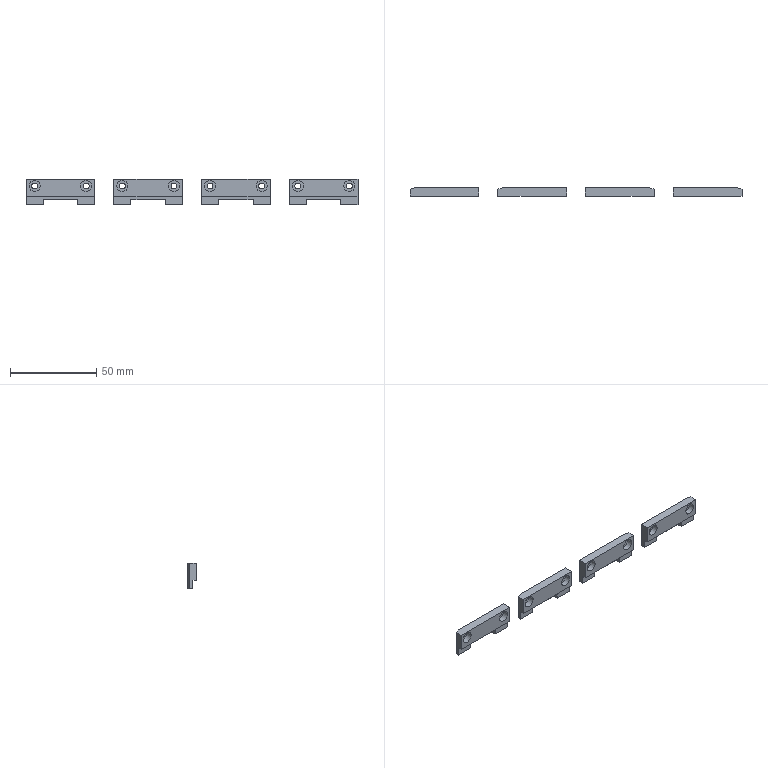CAM job | NX | 3-axis milling | part box 193 x 5 x 15 mm | stock box 198 x 8 x 20 mm
Tools:
number,name,description,diameter,corner_radius,flute_length,length,flutes
6,D6,平底铣刀-粗,6.0,0.0,25.0,75.0,2
9,D10,平底铣刀-粗,10.0,0.0,35.0,75.0,2
7,D6-J,平底铣刀-精,6.0,0.0,25.0,75.0,2
10,D10-J,平底铣刀-精,10.0,0.0,35.0,75.0,2
2,D6-CHAMFER,倒角刀,6.0,0.0,3.0,25.0,2
Operations:
program,operation,operation_type,tool,method,geometry_group,spindle_rpm,surface_speed,feed_per_tooth,feed_cut,feed_plunge,cut_length_mm,path_length_mm,cut_time_min,machine_time_min
A,TOP-FACE,FaceMilling,D10-J,SIDE-FINISH-DEPTHK-STEPG,W-A,4500.0,1385.0,0.1667,1500.0,100.0,217.0,273.0,0.1447,0.1503
A,OUTLINE-ROUGH_2,VolumeBased25DMillingOperation,D10,METHOD,W-A,8000.0,251.327,0.375,6000.0,80.0,10188.726,10637.226,1.698,1.743
A,FLOOR-WALL-LAYER-ROUGH-MID_COPY,VolumeBased25DMillingOperation,D6,LAYER-ROUGH-DEPTHK-STEPG,W-A,8000.0,150.792,0.1875,3000.0,100.0,2411.024,4308.622,0.8037,0.9934
A,FLOOR-WALL-LAYER-ROUGH-MID_COPY_1,VolumeBased25DMillingOperation,D6,LAYER-ROUGH-DEPTHK-STEPG,W-A,8000.0,150.792,0.1875,3000.0,100.0,2153.804,2359.745,0.7179,0.7385
A,SOLID-ONLY,SurfaceContour,D6-CHAMFER,METHOD,W-A,8000.0,150.796,0.1875,3000.0,100.0,565.479,1570.794,0.1885,0.289
A,FLOOR-FINISH_2,VolumeBased25DMillingOperation,D6-J,METHOD,W-A,9000.0,169.646,0.0556,1000.0,100.0,190.0,604.5,0.19,0.2315
A,FLOOR-SIDE-FINISH_3,VolumeBased25DMillingOperation,D6-J,METHOD,W-A,9000.0,169.646,0.0556,1000.0,100.0,198.966,485.726,0.199,0.2276
A,FLOOR-SIDE-FINISH_4,VolumeBased25DMillingOperation,D6-J,METHOD,W-A,9000.0,169.646,0.0556,1000.0,100.0,116.331,773.582,0.1163,0.1821
A,OUTLINE-SEMIFINISH_2,VolumeBased25DMillingOperation,D6-J,METHOD,W-A,9000.0,169.646,0.0556,1000.0,100.0,903.537,1711.068,0.9035,0.9843